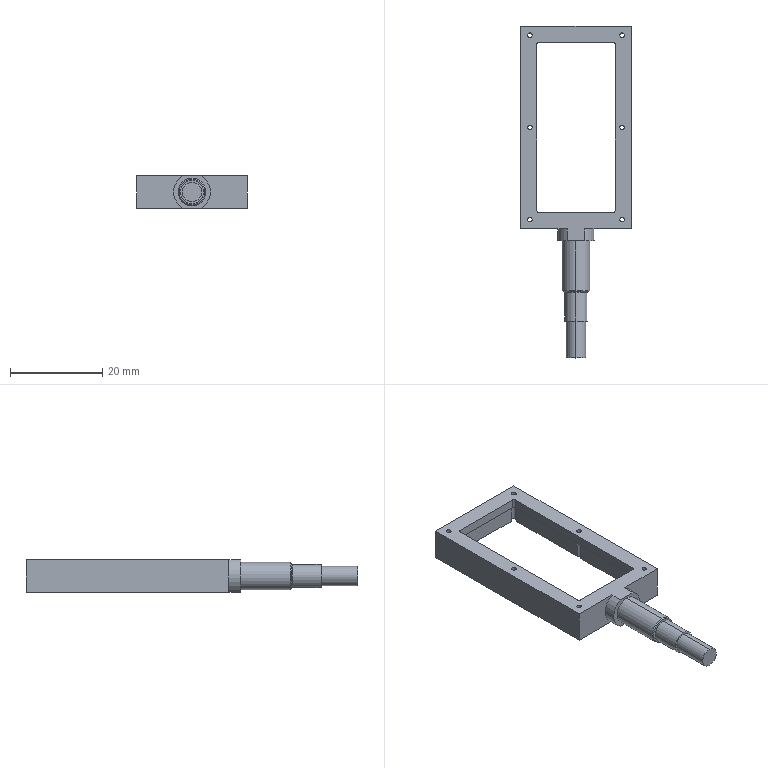Part | 1 solid | 75 faces | box 24 x 72 x 7 mm | volume 2757 mm3 | cylinder 42 | plane 23 | cone 10 | commonest cylinder face diameters 1 x24 1.25 x8 4.2 x2 4.4 x2 5 x2 6 x2